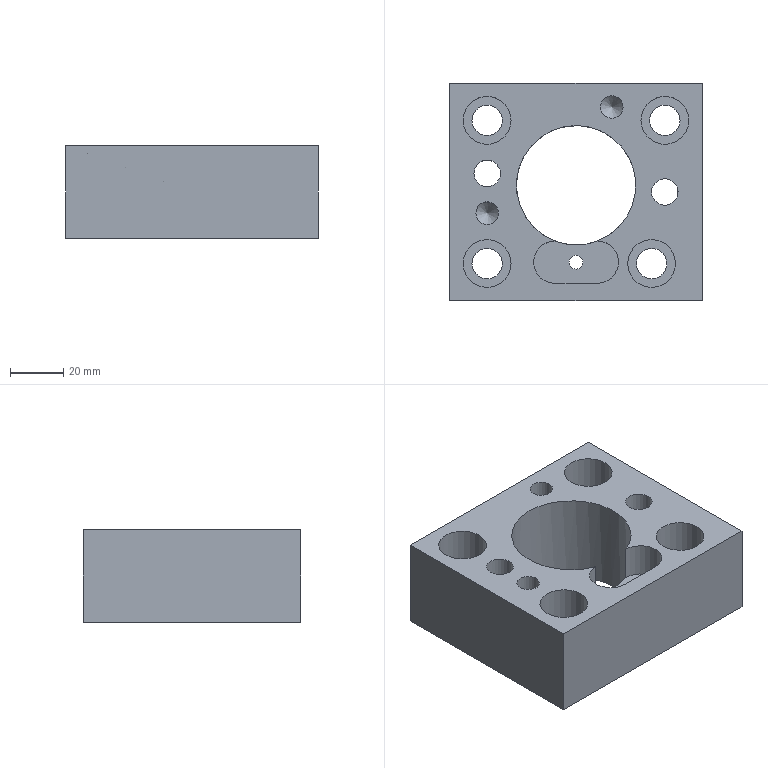Part | STEP file | lll_id4554_x_t | 1 solid | 30 faces | box 95 x 82 x 35 mm | volume 179460 mm3 | cylinder 16 | plane 12 | cone 2 | commonest cylinder face diameters 11.509 x4 18.008 x4 8.506 x2 10 x2 16 x2 5.206 x1
STEP:
#1=CARTESIAN_POINT('',(3213.477,19.288,0.));
#2=VERTEX_POINT('',#1);
#3=CARTESIAN_POINT('',(3213.553,35.287,0.));
#4=VERTEX_POINT('',#3);
#5=CARTESIAN_POINT('',(3213.477,27.288,0.));
#6=DIRECTION('',(0.,0.,1.));
#7=DIRECTION('',(0.,1.,0.));
#8=AXIS2_PLACEMENT_3D('',#5,#6,#7);
#9=CIRCLE('',#8,8.);
#10=EDGE_CURVE('',#2,#4,#9,.T.);
#11=ORIENTED_EDGE('',*,*,#10,.F.);
#12=CARTESIAN_POINT('',(3197.477,19.288,0.));
#13=VERTEX_POINT('',#12);
#14=CARTESIAN_POINT('',(3216.439,19.288,0.));
#15=DIRECTION('',(-1.,0.,0.));
#16=VECTOR('',#15,1.);
#17=LINE('',#14,#16);
#18=EDGE_CURVE('',#2,#13,#17,.T.);
#19=ORIENTED_EDGE('',*,*,#18,.T.);
#20=CARTESIAN_POINT('',(3197.4,35.287,0.));
#21=VERTEX_POINT('',#20);
#22=CARTESIAN_POINT('',(3197.477,27.288,0.));
#23=DIRECTION('',(0.,0.,1.));
#24=DIRECTION('',(0.,1.,0.));
#25=AXIS2_PLACEMENT_3D('',#22,#23,#24);
#26=CIRCLE('',#25,8.);
#27=EDGE_CURVE('',#21,#13,#26,.T.);
#28=ORIENTED_EDGE('',*,*,#27,.F.);
#29=CARTESIAN_POINT('',(3205.477,56.288,0.));
#30=DIRECTION('',(0.,0.,1.));
#31=DIRECTION('',(-1.,0.,0.));
#32=AXIS2_PLACEMENT_3D('',#29,#30,#31);
#33=CIRCLE('',#32,22.5);
#34=EDGE_CURVE('',#4,#21,#33,.T.);
#35=ORIENTED_EDGE('',*,*,#34,.F.);
#36=EDGE_LOOP('',(#11,#19,#28,#35));
#37=FACE_BOUND('',#36,.T.);
#38=CARTESIAN_POINT('',(3180.939,26.75,0.));
#39=VERTEX_POINT('',#38);
#40=CARTESIAN_POINT('',(3171.935,26.75,0.));
#41=DIRECTION('',(0.,0.,-1.));
#42=DIRECTION('',(1.,0.,0.));
#43=AXIS2_PLACEMENT_3D('',#40,#41,#42);
#44=CIRCLE('',#43,9.004);
#45=EDGE_CURVE('',#39,#39,#44,.T.);
#46=ORIENTED_EDGE('',*,*,#45,.T.);
#47=EDGE_LOOP('',(#46));
#48=FACE_BOUND('',#47,.T.);
#49=CARTESIAN_POINT('',(3162.931,80.75,0.));
#50=VERTEX_POINT('',#49);
#51=CARTESIAN_POINT('',(3171.935,80.75,0.));
#52=DIRECTION('',(0.,0.,1.));
#53=DIRECTION('',(-1.,0.,0.));
#54=AXIS2_PLACEMENT_3D('',#51,#52,#53);
#55=CIRCLE('',#54,9.004);
#56=EDGE_CURVE('',#50,#50,#55,.T.);
#57=ORIENTED_EDGE('',*,*,#56,.F.);
#58=EDGE_LOOP('',(#57));
#59=FACE_BOUND('',#58,.T.);
#60=CARTESIAN_POINT('',(3176.188,45.75,0.));
#61=VERTEX_POINT('',#60);
#62=CARTESIAN_POINT('',(3171.935,45.75,0.));
#63=DIRECTION('',(0.,0.,1.));
#64=DIRECTION('',(1.,0.,0.));
#65=AXIS2_PLACEMENT_3D('',#62,#63,#64);
#66=CIRCLE('',#65,4.253);
#67=EDGE_CURVE('',#61,#61,#66,.T.);
#68=ORIENTED_EDGE('',*,*,#67,.F.);
#69=EDGE_LOOP('',(#68));
#70=FACE_BOUND('',#69,.T.);
#71=CARTESIAN_POINT('',(3176.935,60.75,0.));
#72=VERTEX_POINT('',#71);
#73=CARTESIAN_POINT('',(3171.935,60.75,0.));
#74=DIRECTION('',(0.,0.,1.));
#75=DIRECTION('',(1.,0.,0.));
#76=AXIS2_PLACEMENT_3D('',#73,#74,#75);
#77=CIRCLE('',#76,5.);
#78=EDGE_CURVE('',#72,#72,#77,.T.);
#79=ORIENTED_EDGE('',*,*,#78,.F.);
#80=EDGE_LOOP('',(#79));
#81=FACE_BOUND('',#80,.T.);
#82=CARTESIAN_POINT('',(3252.935,94.75,0.));
#83=VERTEX_POINT('',#82);
#84=CARTESIAN_POINT('',(3157.935,94.75,0.));
#85=VERTEX_POINT('',#84);
#86=CARTESIAN_POINT('',(3266.435,94.75,0.));
#87=DIRECTION('',(-1.,0.,0.));
#88=VECTOR('',#87,1.);
#89=LINE('',#86,#88);
#90=EDGE_CURVE('',#83,#85,#89,.T.);
#91=ORIENTED_EDGE('',*,*,#90,.T.);
#92=CARTESIAN_POINT('',(3157.935,12.75,0.));
#93=VERTEX_POINT('',#92);
#94=CARTESIAN_POINT('',(3157.935,215.25,0.));
#95=DIRECTION('',(0.,1.,0.));
#96=VECTOR('',#95,1.);
#97=LINE('',#94,#96);
#98=EDGE_CURVE('',#93,#85,#97,.T.);
#99=ORIENTED_EDGE('',*,*,#98,.F.);
#100=CARTESIAN_POINT('',(3252.935,12.75,0.));
#101=VERTEX_POINT('',#100);
#102=CARTESIAN_POINT('',(3266.435,12.75,0.));
#103=DIRECTION('',(-1.,0.,0.));
#104=VECTOR('',#103,1.);
#105=LINE('',#102,#104);
#106=EDGE_CURVE('',#101,#93,#105,.T.);
#107=ORIENTED_EDGE('',*,*,#106,.F.);
#108=CARTESIAN_POINT('',(3252.935,215.25,0.));
#109=DIRECTION('',(0.,1.,0.));
#110=VECTOR('',#109,1.);
#111=LINE('',#108,#110);
#112=EDGE_CURVE('',#101,#83,#111,.T.);
#113=ORIENTED_EDGE('',*,*,#112,.T.);
#114=EDGE_LOOP('',(#91,#99,#107,#113));
#115=FACE_BOUND('',#114,.T.);
#116=CARTESIAN_POINT('',(3243.935,53.75,0.));
#117=VERTEX_POINT('',#116);
#118=CARTESIAN_POINT('',(3238.935,53.75,0.));
#119=DIRECTION('',(0.,0.,1.));
#120=DIRECTION('',(1.,0.,0.));
#121=AXIS2_PLACEMENT_3D('',#118,#119,#120);
#122=CIRCLE('',#121,5.);
#123=EDGE_CURVE('',#117,#117,#122,.T.);
#124=ORIENTED_EDGE('',*,*,#123,.F.);
#125=EDGE_LOOP('',(#124));
#126=FACE_BOUND('',#125,.T.);
#127=CARTESIAN_POINT('',(3223.188,85.75,0.));
#128=VERTEX_POINT('',#127);
#129=CARTESIAN_POINT('',(3218.935,85.75,0.));
#130=DIRECTION('',(0.,0.,1.));
#131=DIRECTION('',(1.,0.,0.));
#132=AXIS2_PLACEMENT_3D('',#129,#130,#131);
#133=CIRCLE('',#132,4.253);
#134=EDGE_CURVE('',#128,#128,#133,.T.);
#135=ORIENTED_EDGE('',*,*,#134,.F.);
#136=EDGE_LOOP('',(#135));
#137=FACE_BOUND('',#136,.T.);
#138=CARTESIAN_POINT('',(3242.939,26.75,0.));
#139=VERTEX_POINT('',#138);
#140=CARTESIAN_POINT('',(3233.935,26.75,0.));
#141=DIRECTION('',(0.,0.,1.));
#142=DIRECTION('',(1.,0.,0.));
#143=AXIS2_PLACEMENT_3D('',#140,#141,#142);
#144=CIRCLE('',#143,9.004);
#145=EDGE_CURVE('',#139,#139,#144,.T.);
#146=ORIENTED_EDGE('',*,*,#145,.F.);
#147=EDGE_LOOP('',(#146));
#148=FACE_BOUND('',#147,.T.);
#149=CARTESIAN_POINT('',(3247.939,80.75,0.));
#150=VERTEX_POINT('',#149);
#151=CARTESIAN_POINT('',(3238.935,80.75,0.));
#152=DIRECTION('',(0.,0.,-1.));
#153=DIRECTION('',(1.,0.,0.));
#154=AXIS2_PLACEMENT_3D('',#151,#152,#153);
#155=CIRCLE('',#154,9.004);
#156=EDGE_CURVE('',#150,#150,#155,.T.);
#157=ORIENTED_EDGE('',*,*,#156,.T.);
#158=EDGE_LOOP('',(#157));
#159=FACE_BOUND('',#158,.T.);
#160=CARTESIAN_POINT('',(3266.435,215.25,0.));
#161=DIRECTION('',(0.,0.,1.));
#162=DIRECTION('',(-1.,0.,0.));
#163=AXIS2_PLACEMENT_3D('',#160,#161,#162);
#164=PLANE('',#163);
#165=ADVANCED_FACE('',(#37,#48,#59,#70,#81,#115,#126,#137,#148,#159),#164,.T.);
#166=CARTESIAN_POINT('',(3213.553,35.287,-13.));
#167=VERTEX_POINT('',#166);
#168=CARTESIAN_POINT('',(3197.4,35.287,-13.));
#169=VERTEX_POINT('',#168);
#170=CARTESIAN_POINT('',(3205.477,56.288,-13.));
#171=DIRECTION('',(0.,0.,-1.));
#172=DIRECTION('',(1.,0.,0.));
#173=AXIS2_PLACEMENT_3D('',#170,#171,#172);
#174=CIRCLE('',#173,22.5);
#175=EDGE_CURVE('',#167,#169,#174,.T.);
#176=ORIENTED_EDGE('',*,*,#175,.F.);
#177=CARTESIAN_POINT('',(3213.553,35.287,-6.5));
#178=DIRECTION('',(0.,0.,1.));
#179=VECTOR('',#178,1.);
#180=LINE('',#177,#179);
#181=EDGE_CURVE('',#167,#4,#180,.T.);
#182=ORIENTED_EDGE('',*,*,#181,.T.);
#183=ORIENTED_EDGE('',*,*,#34,.T.);
#184=CARTESIAN_POINT('',(3197.4,35.287,-6.5));
#185=DIRECTION('',(0.,0.,-1.));
#186=VECTOR('',#185,1.);
#187=LINE('',#184,#186);
#188=EDGE_CURVE('',#21,#169,#187,.T.);
#189=ORIENTED_EDGE('',*,*,#188,.T.);
#190=EDGE_LOOP('',(#176,#182,#183,#189));
#191=FACE_BOUND('',#190,.T.);
#192=CARTESIAN_POINT('',(3182.977,56.288,-35.));
#193=VERTEX_POINT('',#192);
#194=CARTESIAN_POINT('',(3205.477,56.288,-35.));
#195=DIRECTION('',(0.,0.,-1.));
#196=DIRECTION('',(-1.,0.,0.));
#197=AXIS2_PLACEMENT_3D('',#194,#195,#196);
#198=CIRCLE('',#197,22.5);
#199=EDGE_CURVE('',#193,#193,#198,.T.);
#200=ORIENTED_EDGE('',*,*,#199,.T.);
#201=EDGE_LOOP('',(#200));
#202=FACE_BOUND('',#201,.T.);
#203=CARTESIAN_POINT('',(3205.477,56.288,-15.));
#204=DIRECTION('',(0.,0.,-1.));
#205=DIRECTION('',(0.,-1.,0.));
#206=AXIS2_PLACEMENT_3D('',#203,#204,#205);
#207=CYLINDRICAL_SURFACE('',#206,22.5);
#208=ADVANCED_FACE('',(#191,#202),#207,.F.);
#209=CARTESIAN_POINT('',(3157.935,94.75,-35.));
#210=VERTEX_POINT('',#209);
#211=CARTESIAN_POINT('',(3157.935,94.75,-17.5));
#212=DIRECTION('',(0.,0.,-1.));
#213=VECTOR('',#212,1.);
#214=LINE('',#211,#213);
#215=EDGE_CURVE('',#85,#210,#214,.T.);
#216=ORIENTED_EDGE('',*,*,#215,.T.);
#217=CARTESIAN_POINT('',(3157.935,12.75,-35.));
#218=VERTEX_POINT('',#217);
#219=CARTESIAN_POINT('',(3157.935,215.25,-35.));
#220=DIRECTION('',(0.,-1.,0.));
#221=VECTOR('',#220,1.);
#222=LINE('',#219,#221);
#223=EDGE_CURVE('',#210,#218,#222,.T.);
#224=ORIENTED_EDGE('',*,*,#223,.T.);
#225=CARTESIAN_POINT('',(3157.935,12.75,-32.));
#226=DIRECTION('',(0.,0.,1.));
#227=VECTOR('',#226,1.);
#228=LINE('',#225,#227);
#229=EDGE_CURVE('',#218,#93,#228,.T.);
#230=ORIENTED_EDGE('',*,*,#229,.T.);
#231=ORIENTED_EDGE('',*,*,#98,.T.);
#232=EDGE_LOOP('',(#216,#224,#230,#231));
#233=FACE_OUTER_BOUND('',#232,.T.);
#234=CARTESIAN_POINT('',(3157.935,215.25,-32.));
#235=DIRECTION('',(-1.,0.,0.));
#236=DIRECTION('',(0.,0.,-1.));
#237=AXIS2_PLACEMENT_3D('',#234,#235,#236);
#238=PLANE('',#237);
#239=ADVANCED_FACE('',(#233),#238,.T.);
#240=CARTESIAN_POINT('',(3205.477,24.685,-35.));
#241=VERTEX_POINT('',#240);
#242=CARTESIAN_POINT('',(3205.477,27.288,-35.));
#243=DIRECTION('',(0.,0.,-1.));
#244=DIRECTION('',(0.,-1.,0.));
#245=AXIS2_PLACEMENT_3D('',#242,#243,#244);
#246=CIRCLE('',#245,2.603);
#247=EDGE_CURVE('',#241,#241,#246,.T.);
#248=ORIENTED_EDGE('',*,*,#247,.F.);
#249=EDGE_LOOP('',(#248));
#250=FACE_BOUND('',#249,.T.);
#251=ORIENTED_EDGE('',*,*,#199,.F.);
#252=EDGE_LOOP('',(#251));
#253=FACE_BOUND('',#252,.T.);
#254=CARTESIAN_POINT('',(3233.181,80.75,-35.));
#255=VERTEX_POINT('',#254);
#256=CARTESIAN_POINT('',(3238.935,80.75,-35.));
#257=DIRECTION('',(0.,0.,-1.));
#258=DIRECTION('',(-1.,0.,0.));
#259=AXIS2_PLACEMENT_3D('',#256,#257,#258);
#260=CIRCLE('',#259,5.755);
#261=EDGE_CURVE('',#255,#255,#260,.T.);
#262=ORIENTED_EDGE('',*,*,#261,.F.);
#263=EDGE_LOOP('',(#262));
#264=FACE_BOUND('',#263,.T.);
#265=CARTESIAN_POINT('',(3228.181,26.75,-35.));
#266=VERTEX_POINT('',#265);
#267=CARTESIAN_POINT('',(3233.935,26.75,-35.));
#268=DIRECTION('',(0.,0.,-1.));
#269=DIRECTION('',(-1.,0.,0.));
#270=AXIS2_PLACEMENT_3D('',#267,#268,#269);
#271=CIRCLE('',#270,5.755);
#272=EDGE_CURVE('',#266,#266,#271,.T.);
#273=ORIENTED_EDGE('',*,*,#272,.F.);
#274=EDGE_LOOP('',(#273));
#275=FACE_BOUND('',#274,.T.);
#276=CARTESIAN_POINT('',(3233.935,53.75,-35.));
#277=VERTEX_POINT('',#276);
#278=CARTESIAN_POINT('',(3238.935,53.75,-35.));
#279=DIRECTION('',(0.,0.,-1.));
#280=DIRECTION('',(-1.,0.,0.));
#281=AXIS2_PLACEMENT_3D('',#278,#279,#280);
#282=CIRCLE('',#281,5.);
#283=EDGE_CURVE('',#277,#277,#282,.T.);
#284=ORIENTED_EDGE('',*,*,#283,.F.);
#285=EDGE_LOOP('',(#284));
#286=FACE_BOUND('',#285,.T.);
#287=CARTESIAN_POINT('',(3166.181,26.75,-35.));
#288=VERTEX_POINT('',#287);
#289=CARTESIAN_POINT('',(3171.935,26.75,-35.));
#290=DIRECTION('',(0.,0.,-1.));
#291=DIRECTION('',(-1.,0.,0.));
#292=AXIS2_PLACEMENT_3D('',#289,#290,#291);
#293=CIRCLE('',#292,5.755);
#294=EDGE_CURVE('',#288,#288,#293,.T.);
#295=ORIENTED_EDGE('',*,*,#294,.F.);
#296=EDGE_LOOP('',(#295));
#297=FACE_BOUND('',#296,.T.);
#298=CARTESIAN_POINT('',(3166.181,80.75,-35.));
#299=VERTEX_POINT('',#298);
#300=CARTESIAN_POINT('',(3171.935,80.75,-35.));
#301=DIRECTION('',(0.,0.,-1.));
#302=DIRECTION('',(-1.,0.,0.));
#303=AXIS2_PLACEMENT_3D('',#300,#301,#302);
#304=CIRCLE('',#303,5.755);
#305=EDGE_CURVE('',#299,#299,#304,.T.);
#306=ORIENTED_EDGE('',*,*,#305,.F.);
#307=EDGE_LOOP('',(#306));
#308=FACE_BOUND('',#307,.T.);
#309=CARTESIAN_POINT('',(3166.935,60.75,-35.));
#310=VERTEX_POINT('',#309);
#311=CARTESIAN_POINT('',(3171.935,60.75,-35.));
#312=DIRECTION('',(0.,0.,-1.));
#313=DIRECTION('',(-1.,0.,0.));
#314=AXIS2_PLACEMENT_3D('',#311,#312,#313);
#315=CIRCLE('',#314,5.);
#316=EDGE_CURVE('',#310,#310,#315,.T.);
#317=ORIENTED_EDGE('',*,*,#316,.F.);
#318=EDGE_LOOP('',(#317));
#319=FACE_BOUND('',#318,.T.);
#320=CARTESIAN_POINT('',(3252.935,94.75,-35.));
#321=VERTEX_POINT('',#320);
#322=CARTESIAN_POINT('',(3266.435,94.75,-35.));
#323=DIRECTION('',(-1.,0.,0.));
#324=VECTOR('',#323,1.);
#325=LINE('',#322,#324);
#326=EDGE_CURVE('',#321,#210,#325,.T.);
#327=ORIENTED_EDGE('',*,*,#326,.F.);
#328=CARTESIAN_POINT('',(3252.935,12.75,-35.));
#329=VERTEX_POINT('',#328);
#330=CARTESIAN_POINT('',(3252.935,215.25,-35.));
#331=DIRECTION('',(0.,1.,0.));
#332=VECTOR('',#331,1.);
#333=LINE('',#330,#332);
#334=EDGE_CURVE('',#329,#321,#333,.T.);
#335=ORIENTED_EDGE('',*,*,#334,.F.);
#336=CARTESIAN_POINT('',(3266.435,12.75,-35.));
#337=DIRECTION('',(1.,0.,0.));
#338=VECTOR('',#337,1.);
#339=LINE('',#336,#338);
#340=EDGE_CURVE('',#218,#329,#339,.T.);
#341=ORIENTED_EDGE('',*,*,#340,.F.);
#342=ORIENTED_EDGE('',*,*,#223,.F.);
#343=EDGE_LOOP('',(#327,#335,#341,#342));
#344=FACE_BOUND('',#343,.T.);
#345=CARTESIAN_POINT('',(3266.435,215.25,-35.));
#346=DIRECTION('',(0.,0.,-1.));
#347=DIRECTION('',(1.,0.,0.));
#348=AXIS2_PLACEMENT_3D('',#345,#346,#347);
#349=PLANE('',#348);
#350=ADVANCED_FACE('',(#250,#253,#264,#275,#286,#297,#308,#319,#344),#349,.T.);
#351=CARTESIAN_POINT('',(3252.935,12.75,-32.));
#352=DIRECTION('',(0.,0.,1.));
#353=VECTOR('',#352,1.);
#354=LINE('',#351,#353);
#355=EDGE_CURVE('',#329,#101,#354,.T.);
#356=ORIENTED_EDGE('',*,*,#355,.T.);
#357=ORIENTED_EDGE('',*,*,#106,.T.);
#358=ORIENTED_EDGE('',*,*,#229,.F.);
#359=ORIENTED_EDGE('',*,*,#340,.T.);
#360=EDGE_LOOP('',(#356,#357,#358,#359));
#361=FACE_OUTER_BOUND('',#360,.T.);
#362=CARTESIAN_POINT('',(3266.435,12.75,-32.));
#363=DIRECTION('',(0.,-1.,0.));
#364=DIRECTION('',(0.,0.,1.));
#365=AXIS2_PLACEMENT_3D('',#362,#363,#364);
#366=PLANE('',#365);
#367=ADVANCED_FACE('',(#361),#366,.T.);
#368=ORIENTED_EDGE('',*,*,#334,.T.);
#369=CARTESIAN_POINT('',(3252.935,94.75,-17.5));
#370=DIRECTION('',(0.,0.,1.));
#371=VECTOR('',#370,1.);
#372=LINE('',#369,#371);
#373=EDGE_CURVE('',#321,#83,#372,.T.);
#374=ORIENTED_EDGE('',*,*,#373,.T.);
#375=ORIENTED_EDGE('',*,*,#112,.F.);
#376=ORIENTED_EDGE('',*,*,#355,.F.);
#377=EDGE_LOOP('',(#368,#374,#375,#376));
#378=FACE_OUTER_BOUND('',#377,.T.);
#379=CARTESIAN_POINT('',(3252.935,0.,-17.5));
#380=DIRECTION('',(-1.,0.,0.));
#381=DIRECTION('',(0.,0.,1.));
#382=AXIS2_PLACEMENT_3D('',#379,#380,#381);
#383=PLANE('',#382);
#384=ADVANCED_FACE('',(#378),#383,.F.);
#385=ORIENTED_EDGE('',*,*,#215,.F.);
#386=ORIENTED_EDGE('',*,*,#90,.F.);
#387=ORIENTED_EDGE('',*,*,#373,.F.);
#388=ORIENTED_EDGE('',*,*,#326,.T.);
#389=EDGE_LOOP('',(#385,#386,#387,#388));
#390=FACE_OUTER_BOUND('',#389,.T.);
#391=CARTESIAN_POINT('',(3203.935,94.75,-17.5));
#392=DIRECTION('',(0.,-1.,0.));
#393=DIRECTION('',(0.,0.,-1.));
#394=AXIS2_PLACEMENT_3D('',#391,#392,#393);
#395=PLANE('',#394);
#396=ADVANCED_FACE('',(#390),#395,.F.);
#397=ORIENTED_EDGE('',*,*,#78,.T.);
#398=EDGE_LOOP('',(#397));
#399=FACE_BOUND('',#398,.T.);
#400=ORIENTED_EDGE('',*,*,#316,.T.);
#401=EDGE_LOOP('',(#400));
#402=FACE_BOUND('',#401,.T.);
#403=CARTESIAN_POINT('',(3171.935,60.75,2.));
#404=DIRECTION('',(0.,0.,-1.));
#405=DIRECTION('',(1.,0.,0.));
#406=AXIS2_PLACEMENT_3D('',#403,#404,#405);
#407=CYLINDRICAL_SURFACE('',#406,5.);
#408=ADVANCED_FACE('',(#399,#402),#407,.F.);
#409=ORIENTED_EDGE('',*,*,#67,.T.);
#410=EDGE_LOOP('',(#409));
#411=FACE_BOUND('',#410,.T.);
#412=CARTESIAN_POINT('',(3167.682,45.75,-28.753));
#413=VERTEX_POINT('',#412);
#414=CARTESIAN_POINT('',(3171.935,45.75,-28.753));
#415=DIRECTION('',(0.,0.,1.));
#416=DIRECTION('',(-1.,0.,0.));
#417=AXIS2_PLACEMENT_3D('',#414,#415,#416);
#418=CIRCLE('',#417,4.253);
#419=EDGE_CURVE('',#413,#413,#418,.T.);
#420=ORIENTED_EDGE('',*,*,#419,.F.);
#421=EDGE_LOOP('',(#420));
#422=FACE_BOUND('',#421,.T.);
#423=CARTESIAN_POINT('',(3171.935,45.75,2.));
#424=DIRECTION('',(0.,0.,-1.));
#425=DIRECTION('',(1.,0.,0.));
#426=AXIS2_PLACEMENT_3D('',#423,#424,#425);
#427=CYLINDRICAL_SURFACE('',#426,4.253);
#428=ADVANCED_FACE('',(#411,#422),#427,.F.);
#429=CARTESIAN_POINT('',(3171.935,45.75,-33.006));
#430=VERTEX_POINT('',#429);
#431=VERTEX_LOOP('',#430);
#432=FACE_BOUND('',#431,.T.);
#433=ORIENTED_EDGE('',*,*,#419,.T.);
#434=EDGE_LOOP('',(#433));
#435=FACE_BOUND('',#434,.T.);
#436=CARTESIAN_POINT('',(3171.935,45.75,-28.753));
#437=DIRECTION('',(0.,0.,1.));
#438=DIRECTION('',(1.,0.,0.));
#439=AXIS2_PLACEMENT_3D('',#436,#437,#438);
#440=CONICAL_SURFACE('',#439,4.253,45.);
#441=ADVANCED_FACE('',(#432,#435),#440,.F.);
#442=ORIENTED_EDGE('',*,*,#305,.T.);
#443=EDGE_LOOP('',(#442));
#444=FACE_BOUND('',#443,.T.);
#445=CARTESIAN_POINT('',(3177.69,80.75,-13.));
#446=VERTEX_POINT('',#445);
#447=CARTESIAN_POINT('',(3171.935,80.75,-13.));
#448=DIRECTION('',(0.,0.,1.));
#449=DIRECTION('',(1.,0.,0.));
#450=AXIS2_PLACEMENT_3D('',#447,#448,#449);
#451=CIRCLE('',#450,5.755);
#452=EDGE_CURVE('',#446,#446,#451,.T.);
#453=ORIENTED_EDGE('',*,*,#452,.T.);
#454=EDGE_LOOP('',(#453));
#455=FACE_BOUND('',#454,.T.);
#456=CARTESIAN_POINT('',(3171.935,80.75,2.));
#457=DIRECTION('',(0.,0.,-1.));
#458=DIRECTION('',(-1.,0.,0.));
#459=AXIS2_PLACEMENT_3D('',#456,#457,#458);
#460=CYLINDRICAL_SURFACE('',#459,5.755);
#461=ADVANCED_FACE('',(#444,#455),#460,.F.);
#462=ORIENTED_EDGE('',*,*,#452,.F.);
#463=EDGE_LOOP('',(#462));
#464=FACE_BOUND('',#463,.T.);
#465=CARTESIAN_POINT('',(3162.931,80.75,-13.));
#466=VERTEX_POINT('',#465);
#467=CARTESIAN_POINT('',(3171.935,80.75,-13.));
#468=DIRECTION('',(0.,0.,1.));
#469=DIRECTION('',(-1.,0.,0.));
#470=AXIS2_PLACEMENT_3D('',#467,#468,#469);
#471=CIRCLE('',#470,9.004);
#472=EDGE_CURVE('',#466,#466,#471,.T.);
#473=ORIENTED_EDGE('',*,*,#472,.T.);
#474=EDGE_LOOP('',(#473));
#475=FACE_BOUND('',#474,.T.);
#476=CARTESIAN_POINT('',(3171.935,80.75,-13.));
#477=DIRECTION('',(0.,0.,-1.));
#478=DIRECTION('',(1.,0.,0.));
#479=AXIS2_PLACEMENT_3D('',#476,#477,#478);
#480=PLANE('',#479);
#481=ADVANCED_FACE('',(#464,#475),#480,.F.);
#482=ORIENTED_EDGE('',*,*,#472,.F.);
#483=EDGE_LOOP('',(#482));
#484=FACE_BOUND('',#483,.T.);
#485=ORIENTED_EDGE('',*,*,#56,.T.);
#486=EDGE_LOOP('',(#485));
#487=FACE_BOUND('',#486,.T.);
#488=CARTESIAN_POINT('',(3171.935,80.75,0.));
#489=DIRECTION('',(0.,0.,-1.));
#490=DIRECTION('',(-1.,0.,0.));
#491=AXIS2_PLACEMENT_3D('',#488,#489,#490);
#492=CYLINDRICAL_SURFACE('',#491,9.004);
#493=ADVANCED_FACE('',(#484,#487),#492,.F.);
#494=ORIENTED_EDGE('',*,*,#294,.T.);
#495=EDGE_LOOP('',(#494));
#496=FACE_BOUND('',#495,.T.);
#497=CARTESIAN_POINT('',(3166.181,26.75,-13.));
#498=VERTEX_POINT('',#497);
#499=CARTESIAN_POINT('',(3171.935,26.75,-13.));
#500=DIRECTION('',(0.,0.,-1.));
#501=DIRECTION('',(-1.,0.,0.));
#502=AXIS2_PLACEMENT_3D('',#499,#500,#501);
#503=CIRCLE('',#502,5.755);
#504=EDGE_CURVE('',#498,#498,#503,.T.);
#505=ORIENTED_EDGE('',*,*,#504,.F.);
#506=EDGE_LOOP('',(#505));
#507=FACE_BOUND('',#506,.T.);
#508=CARTESIAN_POINT('',(3171.935,26.75,2.));
#509=DIRECTION('',(0.,0.,-1.));
#510=DIRECTION('',(1.,0.,0.));
#511=AXIS2_PLACEMENT_3D('',#508,#509,#510);
#512=CYLINDRICAL_SURFACE('',#511,5.755);
#513=ADVANCED_FACE('',(#496,#507),#512,.F.);
#514=ORIENTED_EDGE('',*,*,#504,.T.);
#515=EDGE_LOOP('',(#514));
#516=FACE_BOUND('',#515,.T.);
#517=CARTESIAN_POINT('',(3180.939,26.75,-13.));
#518=VERTEX_POINT('',#517);
#519=CARTESIAN_POINT('',(3171.935,26.75,-13.));
#520=DIRECTION('',(0.,0.,-1.));
#521=DIRECTION('',(1.,0.,0.));
#522=AXIS2_PLACEMENT_3D('',#519,#520,#521);
#523=CIRCLE('',#522,9.004);
#524=EDGE_CURVE('',#518,#518,#523,.T.);
#525=ORIENTED_EDGE('',*,*,#524,.F.);
#526=EDGE_LOOP('',(#525));
#527=FACE_BOUND('',#526,.T.);
#528=CARTESIAN_POINT('',(3171.935,26.75,-13.));
#529=DIRECTION('',(0.,0.,-1.));
#530=DIRECTION('',(-1.,0.,0.));
#531=AXIS2_PLACEMENT_3D('',#528,#529,#530);
#532=PLANE('',#531);
#533=ADVANCED_FACE('',(#516,#527),#532,.F.);
#534=ORIENTED_EDGE('',*,*,#524,.T.);
#535=EDGE_LOOP('',(#534));
#536=FACE_BOUND('',#535,.T.);
#537=ORIENTED_EDGE('',*,*,#45,.F.);
#538=EDGE_LOOP('',(#537));
#539=FACE_BOUND('',#538,.T.);
#540=CARTESIAN_POINT('',(3171.935,26.75,0.));
#541=DIRECTION('',(0.,0.,-1.));
#542=DIRECTION('',(1.,0.,0.));
#543=AXIS2_PLACEMENT_3D('',#540,#541,#542);
#544=CYLINDRICAL_SURFACE('',#543,9.004);
#545=ADVANCED_FACE('',(#536,#539),#544,.F.);
#546=ORIENTED_EDGE('',*,*,#123,.T.);
#547=EDGE_LOOP('',(#546));
#548=FACE_BOUND('',#547,.T.);
#549=ORIENTED_EDGE('',*,*,#283,.T.);
#550=EDGE_LOOP('',(#549));
#551=FACE_BOUND('',#550,.T.);
#552=CARTESIAN_POINT('',(3238.935,53.75,2.));
#553=DIRECTION('',(0.,0.,-1.));
#554=DIRECTION('',(1.,0.,0.));
#555=AXIS2_PLACEMENT_3D('',#552,#553,#554);
#556=CYLINDRICAL_SURFACE('',#555,5.);
#557=ADVANCED_FACE('',(#548,#551),#556,.F.);
#558=ORIENTED_EDGE('',*,*,#134,.T.);
#559=EDGE_LOOP('',(#558));
#560=FACE_BOUND('',#559,.T.);
#561=CARTESIAN_POINT('',(3214.682,85.75,-28.753));
#562=VERTEX_POINT('',#561);
#563=CARTESIAN_POINT('',(3218.935,85.75,-28.753));
#564=DIRECTION('',(0.,0.,1.));
#565=DIRECTION('',(-1.,0.,0.));
#566=AXIS2_PLACEMENT_3D('',#563,#564,#565);
#567=CIRCLE('',#566,4.253);
#568=EDGE_CURVE('',#562,#562,#567,.T.);
#569=ORIENTED_EDGE('',*,*,#568,.F.);
#570=EDGE_LOOP('',(#569));
#571=FACE_BOUND('',#570,.T.);
#572=CARTESIAN_POINT('',(3218.935,85.75,2.));
#573=DIRECTION('',(0.,0.,-1.));
#574=DIRECTION('',(1.,0.,0.));
#575=AXIS2_PLACEMENT_3D('',#572,#573,#574);
#576=CYLINDRICAL_SURFACE('',#575,4.253);
#577=ADVANCED_FACE('',(#560,#571),#576,.F.);
#578=CARTESIAN_POINT('',(3218.935,85.75,-33.006));
#579=VERTEX_POINT('',#578);
#580=VERTEX_LOOP('',#579);
#581=FACE_BOUND('',#580,.T.);
#582=ORIENTED_EDGE('',*,*,#568,.T.);
#583=EDGE_LOOP('',(#582));
#584=FACE_BOUND('',#583,.T.);
#585=CARTESIAN_POINT('',(3218.935,85.75,-28.753));
#586=DIRECTION('',(0.,0.,1.));
#587=DIRECTION('',(1.,0.,0.));
#588=AXIS2_PLACEMENT_3D('',#585,#586,#587);
#589=CONICAL_SURFACE('',#588,4.253,45.);
#590=ADVANCED_FACE('',(#581,#584),#589,.F.);
#591=ORIENTED_EDGE('',*,*,#272,.T.);
#592=EDGE_LOOP('',(#591));
#593=FACE_BOUND('',#592,.T.);
#594=CARTESIAN_POINT('',(3228.181,26.75,-13.));
#595=VERTEX_POINT('',#594);
#596=CARTESIAN_POINT('',(3233.935,26.75,-13.));
#597=DIRECTION('',(0.,0.,1.));
#598=DIRECTION('',(-1.,0.,0.));
#599=AXIS2_PLACEMENT_3D('',#596,#597,#598);
#600=CIRCLE('',#599,5.755);
#601=EDGE_CURVE('',#595,#595,#600,.T.);
#602=ORIENTED_EDGE('',*,*,#601,.T.);
#603=EDGE_LOOP('',(#602));
#604=FACE_BOUND('',#603,.T.);
#605=CARTESIAN_POINT('',(3233.935,26.75,2.));
#606=DIRECTION('',(0.,0.,-1.));
#607=DIRECTION('',(1.,0.,0.));
#608=AXIS2_PLACEMENT_3D('',#605,#606,#607);
#609=CYLINDRICAL_SURFACE('',#608,5.755);
#610=ADVANCED_FACE('',(#593,#604),#609,.F.);
#611=ORIENTED_EDGE('',*,*,#601,.F.);
#612=EDGE_LOOP('',(#611));
#613=FACE_BOUND('',#612,.T.);
#614=CARTESIAN_POINT('',(3242.939,26.75,-13.));
#615=VERTEX_POINT('',#614);
#616=CARTESIAN_POINT('',(3233.935,26.75,-13.));
#617=DIRECTION('',(0.,0.,1.));
#618=DIRECTION('',(1.,0.,0.));
#619=AXIS2_PLACEMENT_3D('',#616,#617,#618);
#620=CIRCLE('',#619,9.004);
#621=EDGE_CURVE('',#615,#615,#620,.T.);
#622=ORIENTED_EDGE('',*,*,#621,.T.);
#623=EDGE_LOOP('',(#622));
#624=FACE_BOUND('',#623,.T.);
#625=CARTESIAN_POINT('',(3233.935,26.75,-13.));
#626=DIRECTION('',(0.,0.,-1.));
#627=DIRECTION('',(-1.,0.,0.));
#628=AXIS2_PLACEMENT_3D('',#625,#626,#627);
#629=PLANE('',#628);
#630=ADVANCED_FACE('',(#613,#624),#629,.F.);
#631=ORIENTED_EDGE('',*,*,#621,.F.);
#632=EDGE_LOOP('',(#631));
#633=FACE_BOUND('',#632,.T.);
#634=ORIENTED_EDGE('',*,*,#145,.T.);
#635=EDGE_LOOP('',(#634));
#636=FACE_BOUND('',#635,.T.);
#637=CARTESIAN_POINT('',(3233.935,26.75,0.));
#638=DIRECTION('',(0.,0.,-1.));
#639=DIRECTION('',(1.,0.,0.));
#640=AXIS2_PLACEMENT_3D('',#637,#638,#639);
#641=CYLINDRICAL_SURFACE('',#640,9.004);
#642=ADVANCED_FACE('',(#633,#636),#641,.F.);
#643=ORIENTED_EDGE('',*,*,#261,.T.);
#644=EDGE_LOOP('',(#643));
#645=FACE_BOUND('',#644,.T.);
#646=CARTESIAN_POINT('',(3233.181,80.75,-13.));
#647=VERTEX_POINT('',#646);
#648=CARTESIAN_POINT('',(3238.935,80.75,-13.));
#649=DIRECTION('',(0.,0.,-1.));
#650=DIRECTION('',(-1.,0.,0.));
#651=AXIS2_PLACEMENT_3D('',#648,#649,#650);
#652=CIRCLE('',#651,5.755);
#653=EDGE_CURVE('',#647,#647,#652,.T.);
#654=ORIENTED_EDGE('',*,*,#653,.F.);
#655=EDGE_LOOP('',(#654));
#656=FACE_BOUND('',#655,.T.);
#657=CARTESIAN_POINT('',(3238.935,80.75,2.));
#658=DIRECTION('',(0.,0.,-1.));
#659=DIRECTION('',(1.,0.,0.));
#660=AXIS2_PLACEMENT_3D('',#657,#658,#659);
#661=CYLINDRICAL_SURFACE('',#660,5.755);
#662=ADVANCED_FACE('',(#645,#656),#661,.F.);
#663=ORIENTED_EDGE('',*,*,#653,.T.);
#664=EDGE_LOOP('',(#663));
#665=FACE_BOUND('',#664,.T.);
#666=CARTESIAN_POINT('',(3247.939,80.75,-13.));
#667=VERTEX_POINT('',#666);
#668=CARTESIAN_POINT('',(3238.935,80.75,-13.));
#669=DIRECTION('',(0.,0.,-1.));
#670=DIRECTION('',(1.,0.,0.));
#671=AXIS2_PLACEMENT_3D('',#668,#669,#670);
#672=CIRCLE('',#671,9.004);
#673=EDGE_CURVE('',#667,#667,#672,.T.);
#674=ORIENTED_EDGE('',*,*,#673,.F.);
#675=EDGE_LOOP('',(#674));
#676=FACE_BOUND('',#675,.T.);
#677=CARTESIAN_POINT('',(3238.935,80.75,-13.));
#678=DIRECTION('',(0.,0.,-1.));
#679=DIRECTION('',(-1.,0.,0.));
#680=AXIS2_PLACEMENT_3D('',#677,#678,#679);
#681=PLANE('',#680);
#682=ADVANCED_FACE('',(#665,#676),#681,.F.);
#683=ORIENTED_EDGE('',*,*,#673,.T.);
#684=EDGE_LOOP('',(#683));
#685=FACE_BOUND('',#684,.T.);
#686=ORIENTED_EDGE('',*,*,#156,.F.);
#687=EDGE_LOOP('',(#686));
#688=FACE_BOUND('',#687,.T.);
#689=CARTESIAN_POINT('',(3238.935,80.75,0.));
#690=DIRECTION('',(0.,0.,-1.));
#691=DIRECTION('',(1.,0.,0.));
#692=AXIS2_PLACEMENT_3D('',#689,#690,#691);
#693=CYLINDRICAL_SURFACE('',#692,9.004);
#694=ADVANCED_FACE('',(#685,#688),#693,.F.);
#695=CARTESIAN_POINT('',(3213.477,19.288,-13.));
#696=VERTEX_POINT('',#695);
#697=CARTESIAN_POINT('',(3213.477,27.288,-13.));
#698=DIRECTION('',(0.,0.,-1.));
#699=DIRECTION('',(0.,1.,0.));
#700=AXIS2_PLACEMENT_3D('',#697,#698,#699);
#701=CIRCLE('',#700,8.);
#702=EDGE_CURVE('',#167,#696,#701,.T.);
#703=ORIENTED_EDGE('',*,*,#702,.T.);
#704=CARTESIAN_POINT('',(3213.477,19.288,-1.));
#705=DIRECTION('',(0.,0.,1.));
#706=VECTOR('',#705,1.);
#707=LINE('',#704,#706);
#708=EDGE_CURVE('',#696,#2,#707,.T.);
#709=ORIENTED_EDGE('',*,*,#708,.T.);
#710=ORIENTED_EDGE('',*,*,#10,.T.);
#711=ORIENTED_EDGE('',*,*,#181,.F.);
#712=EDGE_LOOP('',(#703,#709,#710,#711));
#713=FACE_OUTER_BOUND('',#712,.T.);
#714=CARTESIAN_POINT('',(3213.477,27.288,-1.));
#715=DIRECTION('',(0.,0.,-1.));
#716=DIRECTION('',(0.,1.,0.));
#717=AXIS2_PLACEMENT_3D('',#714,#715,#716);
#718=CYLINDRICAL_SURFACE('',#717,8.);
#719=ADVANCED_FACE('',(#713),#718,.F.);
#720=CARTESIAN_POINT('',(3205.477,29.891,-13.));
#721=VERTEX_POINT('',#720);
#722=CARTESIAN_POINT('',(3205.477,27.288,-13.));
#723=DIRECTION('',(0.,0.,-1.));
#724=DIRECTION('',(0.,1.,0.));
#725=AXIS2_PLACEMENT_3D('',#722,#723,#724);
#726=CIRCLE('',#725,2.603);
#727=EDGE_CURVE('',#721,#721,#726,.T.);
#728=ORIENTED_EDGE('',*,*,#727,.T.);
#729=EDGE_LOOP('',(#728));
#730=FACE_BOUND('',#729,.T.);
#731=ORIENTED_EDGE('',*,*,#175,.T.);
#732=CARTESIAN_POINT('',(3197.477,19.288,-13.));
#733=VERTEX_POINT('',#732);
#734=CARTESIAN_POINT('',(3197.477,27.288,-13.));
#735=DIRECTION('',(0.,0.,-1.));
#736=DIRECTION('',(0.,1.,0.));
#737=AXIS2_PLACEMENT_3D('',#734,#735,#736);
#738=CIRCLE('',#737,8.);
#739=EDGE_CURVE('',#733,#169,#738,.T.);
#740=ORIENTED_EDGE('',*,*,#739,.F.);
#741=CARTESIAN_POINT('',(3197.477,19.288,-13.));
#742=DIRECTION('',(-1.,0.,0.));
#743=VECTOR('',#742,1.);
#744=LINE('',#741,#743);
#745=EDGE_CURVE('',#696,#733,#744,.T.);
#746=ORIENTED_EDGE('',*,*,#745,.F.);
#747=ORIENTED_EDGE('',*,*,#702,.F.);
#748=EDGE_LOOP('',(#731,#740,#746,#747));
#749=FACE_BOUND('',#748,.T.);
#750=CARTESIAN_POINT('',(3197.477,27.288,-13.));
#751=DIRECTION('',(0.,0.,1.));
#752=DIRECTION('',(0.,1.,0.));
#753=AXIS2_PLACEMENT_3D('',#750,#751,#752);
#754=PLANE('',#753);
#755=ADVANCED_FACE('',(#730,#749),#754,.T.);
#756=ORIENTED_EDGE('',*,*,#27,.T.);
#757=CARTESIAN_POINT('',(3197.477,19.288,-1.));
#758=DIRECTION('',(0.,0.,-1.));
#759=VECTOR('',#758,1.);
#760=LINE('',#757,#759);
#761=EDGE_CURVE('',#13,#733,#760,.T.);
#762=ORIENTED_EDGE('',*,*,#761,.T.);
#763=ORIENTED_EDGE('',*,*,#739,.T.);
#764=ORIENTED_EDGE('',*,*,#188,.F.);
#765=EDGE_LOOP('',(#756,#762,#763,#764));
#766=FACE_OUTER_BOUND('',#765,.T.);
#767=CARTESIAN_POINT('',(3197.477,27.288,-1.));
#768=DIRECTION('',(0.,0.,-1.));
#769=DIRECTION('',(0.,1.,0.));
#770=AXIS2_PLACEMENT_3D('',#767,#768,#769);
#771=CYLINDRICAL_SURFACE('',#770,8.);
#772=ADVANCED_FACE('',(#766),#771,.F.);
#773=ORIENTED_EDGE('',*,*,#247,.T.);
#774=EDGE_LOOP('',(#773));
#775=FACE_BOUND('',#774,.T.);
#776=ORIENTED_EDGE('',*,*,#727,.F.);
#777=EDGE_LOOP('',(#776));
#778=FACE_BOUND('',#777,.T.);
#779=CARTESIAN_POINT('',(3205.477,27.288,-13.));
#780=DIRECTION('',(0.,0.,-1.));
#781=DIRECTION('',(0.,1.,0.));
#782=AXIS2_PLACEMENT_3D('',#779,#780,#781);
#783=CYLINDRICAL_SURFACE('',#782,2.603);
#784=ADVANCED_FACE('',(#775,#778),#783,.F.);
#785=ORIENTED_EDGE('',*,*,#18,.F.);
#786=ORIENTED_EDGE('',*,*,#708,.F.);
#787=ORIENTED_EDGE('',*,*,#745,.T.);
#788=ORIENTED_EDGE('',*,*,#761,.F.);
#789=EDGE_LOOP('',(#785,#786,#787,#788));
#790=FACE_OUTER_BOUND('',#789,.T.);
#791=CARTESIAN_POINT('',(2858.057,19.288,0.));
#792=DIRECTION('',(0.,-1.,0.));
#793=DIRECTION('',(0.,0.,1.));
#794=AXIS2_PLACEMENT_3D('',#791,#792,#793);
#795=PLANE('',#794);
#796=ADVANCED_FACE('',(#790),#795,.F.);
#797=CLOSED_SHELL('',(#165,#208,#239,#350,#367,#384,#396,#408,#428,#441,#461,#481,#493,#513,#533,#545,#557,#577,#590,#610,#630,#642,#662,#682,#694,#719,#755,#772,#784,#796));
#798=MANIFOLD_SOLID_BREP('',#797);
#799=(LENGTH_UNIT()NAMED_UNIT(*)SI_UNIT(.MILLI.,.METRE.));
#800=UNCERTAINTY_MEASURE_WITH_UNIT(LENGTH_MEASURE(0.00002),#799,'','');
#801=(NAMED_UNIT(*)PLANE_ANGLE_UNIT()SI_UNIT($,.RADIAN.));
#802=PLANE_ANGLE_MEASURE_WITH_UNIT(PLANE_ANGLE_MEASURE(0.01745),#801);
#803=DIMENSIONAL_EXPONENTS(0.,0.,0.,0.,0.,0.,0.);
#804=(CONVERSION_BASED_UNIT('DEGREE',#802)NAMED_UNIT(#803)PLANE_ANGLE_UNIT());
#805=(NAMED_UNIT(*)SI_UNIT($,.STERADIAN.)SOLID_ANGLE_UNIT());
#806=(GEOMETRIC_REPRESENTATION_CONTEXT(3)GLOBAL_UNCERTAINTY_ASSIGNED_CONTEXT((#800))GLOBAL_UNIT_ASSIGNED_CONTEXT((#799,#804,#805))REPRESENTATION_CONTEXT('',''));
#807=ADVANCED_BREP_SHAPE_REPRESENTATION('',(#798),#806);